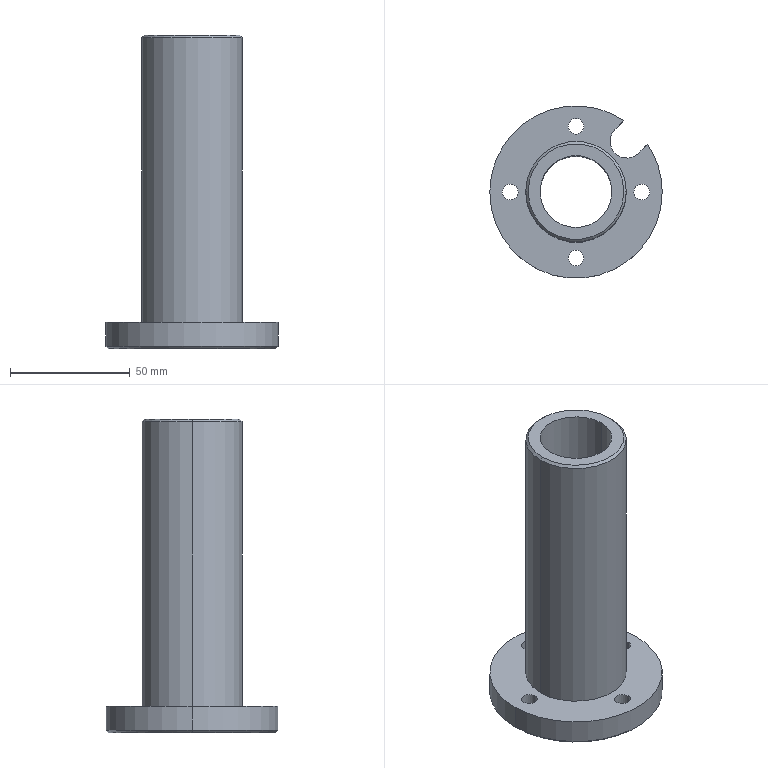Part | SolidWorks | features HoleWzd 2, Revolution 2, Chamfer 1, ICE 1 | 1 solid | 40 faces | box 72 x 72 x 131 mm | volume 113425 mm3 | cylinder 24 | plane 9 | cone 7 | commonest cylinder face diameters 6.6 x8 11 x8 72 x3 30 x2 42 x2 14 x1
STEP:
#1=CARTESIAN_POINT('',(-35.,0.,0.));
#2=VERTEX_POINT('',#1);
#3=CARTESIAN_POINT('',(19.299,29.198,0.));
#4=VERTEX_POINT('',#3);
#5=CARTESIAN_POINT('',(0.,0.,0.));
#6=DIRECTION('',(0.,0.,-1.));
#7=DIRECTION('',(-1.,0.,0.));
#8=AXIS2_PLACEMENT_3D('',#5,#6,#7);
#9=CIRCLE('',#8,35.);
#10=EDGE_CURVE('',#2,#4,#9,.T.);
#11=ORIENTED_EDGE('',*,*,#10,.F.);
#12=CARTESIAN_POINT('',(-36.,0.,1.));
#13=VERTEX_POINT('',#12);
#14=CARTESIAN_POINT('',(-35.,0.,0.));
#15=DIRECTION('',(-0.7071,0.,0.7071));
#16=VECTOR('',#15,1000.);
#17=LINE('',#14,#16);
#18=EDGE_CURVE('',#2,#13,#17,.T.);
#19=ORIENTED_EDGE('',*,*,#18,.T.);
#20=CARTESIAN_POINT('',(20.02,29.92,1.));
#21=VERTEX_POINT('',#20);
#22=CARTESIAN_POINT('',(0.,0.,1.));
#23=DIRECTION('',(0.,0.,1.));
#24=DIRECTION('',(-1.,0.,0.));
#25=AXIS2_PLACEMENT_3D('',#22,#23,#24);
#26=CIRCLE('',#25,36.);
#27=EDGE_CURVE('',#21,#13,#26,.T.);
#28=ORIENTED_EDGE('',*,*,#27,.F.);
#29=CARTESIAN_POINT('',(19.299,29.198,0.));
#30=CARTESIAN_POINT('',(19.539,29.439,0.3332));
#31=CARTESIAN_POINT('',(19.78,29.679,0.6666));
#32=CARTESIAN_POINT('',(20.02,29.92,1.));
#33=B_SPLINE_CURVE_WITH_KNOTS('',3,(#29,#30,#31,#32),.UNSPECIFIED.,.F.,.F.,(4,4),(0.,0.001428),.UNSPECIFIED.);
#34=EDGE_CURVE('',#4,#21,#33,.T.);
#35=ORIENTED_EDGE('',*,*,#34,.F.);
#36=EDGE_LOOP('',(#11,#19,#28,#35));
#37=FACE_OUTER_BOUND('',#36,.T.);
#38=CARTESIAN_POINT('',(0.,0.,0.));
#39=DIRECTION('',(0.,0.,1.));
#40=DIRECTION('',(1.,0.,0.));
#41=AXIS2_PLACEMENT_3D('',#38,#39,#40);
#42=CONICAL_SURFACE('',#41,35.,0.7854);
#43=ADVANCED_FACE('',(#37),#42,.T.);
#44=ORIENTED_EDGE('',*,*,#18,.F.);
#45=CARTESIAN_POINT('',(35.,0.,0.));
#46=VERTEX_POINT('',#45);
#47=CARTESIAN_POINT('',(0.,0.,0.));
#48=DIRECTION('',(0.,0.,-1.));
#49=DIRECTION('',(-1.,0.,0.));
#50=AXIS2_PLACEMENT_3D('',#47,#48,#49);
#51=CIRCLE('',#50,35.);
#52=EDGE_CURVE('',#46,#2,#51,.T.);
#53=ORIENTED_EDGE('',*,*,#52,.F.);
#54=CARTESIAN_POINT('',(36.,0.,1.));
#55=VERTEX_POINT('',#54);
#56=CARTESIAN_POINT('',(35.,0.,0.));
#57=DIRECTION('',(0.7071,0.,0.7071));
#58=VECTOR('',#57,1000.);
#59=LINE('',#56,#58);
#60=EDGE_CURVE('',#46,#55,#59,.T.);
#61=ORIENTED_EDGE('',*,*,#60,.T.);
#62=CARTESIAN_POINT('',(0.,0.,1.));
#63=DIRECTION('',(0.,0.,1.));
#64=DIRECTION('',(-1.,0.,0.));
#65=AXIS2_PLACEMENT_3D('',#62,#63,#64);
#66=CIRCLE('',#65,36.);
#67=EDGE_CURVE('',#13,#55,#66,.T.);
#68=ORIENTED_EDGE('',*,*,#67,.F.);
#69=EDGE_LOOP('',(#44,#53,#61,#68));
#70=FACE_OUTER_BOUND('',#69,.T.);
#71=CARTESIAN_POINT('',(0.,0.,0.));
#72=DIRECTION('',(0.,0.,1.));
#73=DIRECTION('',(1.,0.,0.));
#74=AXIS2_PLACEMENT_3D('',#71,#72,#73);
#75=CONICAL_SURFACE('',#74,35.,0.7854);
#76=ADVANCED_FACE('',(#70),#75,.T.);
#77=CARTESIAN_POINT('',(20.,0.,131.));
#78=VERTEX_POINT('',#77);
#79=CARTESIAN_POINT('',(-20.,0.,131.));
#80=VERTEX_POINT('',#79);
#81=CARTESIAN_POINT('',(0.,0.,131.));
#82=DIRECTION('',(0.,0.,1.));
#83=DIRECTION('',(1.,0.,0.));
#84=AXIS2_PLACEMENT_3D('',#81,#82,#83);
#85=CIRCLE('',#84,20.);
#86=EDGE_CURVE('',#78,#80,#85,.T.);
#87=ORIENTED_EDGE('',*,*,#86,.F.);
#88=CARTESIAN_POINT('',(21.,0.,130.));
#89=VERTEX_POINT('',#88);
#90=CARTESIAN_POINT('',(21.,0.,130.));
#91=DIRECTION('',(0.7071,0.,-0.7071));
#92=VECTOR('',#91,1000.);
#93=LINE('',#90,#92);
#94=EDGE_CURVE('',#78,#89,#93,.T.);
#95=ORIENTED_EDGE('',*,*,#94,.T.);
#96=CARTESIAN_POINT('',(-21.,0.,130.));
#97=VERTEX_POINT('',#96);
#98=CARTESIAN_POINT('',(0.,0.,130.));
#99=DIRECTION('',(0.,0.,-1.));
#100=DIRECTION('',(1.,0.,0.));
#101=AXIS2_PLACEMENT_3D('',#98,#99,#100);
#102=CIRCLE('',#101,21.);
#103=EDGE_CURVE('',#97,#89,#102,.T.);
#104=ORIENTED_EDGE('',*,*,#103,.F.);
#105=CARTESIAN_POINT('',(-21.,0.,130.));
#106=DIRECTION('',(-0.7071,0.,-0.7071));
#107=VECTOR('',#106,1000.);
#108=LINE('',#105,#107);
#109=EDGE_CURVE('',#80,#97,#108,.T.);
#110=ORIENTED_EDGE('',*,*,#109,.F.);
#111=EDGE_LOOP('',(#87,#95,#104,#110));
#112=FACE_OUTER_BOUND('',#111,.T.);
#113=CARTESIAN_POINT('',(0.,0.,130.));
#114=DIRECTION('',(0.,0.,-1.));
#115=DIRECTION('',(-1.,0.,0.));
#116=AXIS2_PLACEMENT_3D('',#113,#114,#115);
#117=CONICAL_SURFACE('',#116,21.,0.7854);
#118=ADVANCED_FACE('',(#112),#117,.T.);
#119=CARTESIAN_POINT('',(15.,0.,1.));
#120=VERTEX_POINT('',#119);
#121=CARTESIAN_POINT('',(-15.,0.,1.));
#122=VERTEX_POINT('',#121);
#123=CARTESIAN_POINT('',(0.,0.,1.));
#124=DIRECTION('',(0.,0.,-1.));
#125=DIRECTION('',(-1.,0.,0.));
#126=AXIS2_PLACEMENT_3D('',#123,#124,#125);
#127=CIRCLE('',#126,15.);
#128=EDGE_CURVE('',#120,#122,#127,.T.);
#129=ORIENTED_EDGE('',*,*,#128,.F.);
#130=CARTESIAN_POINT('',(16.,0.,0.));
#131=VERTEX_POINT('',#130);
#132=CARTESIAN_POINT('',(15.,0.,1.));
#133=DIRECTION('',(0.7071,0.,-0.7071));
#134=VECTOR('',#133,1000.);
#135=LINE('',#132,#134);
#136=EDGE_CURVE('',#120,#131,#135,.T.);
#137=ORIENTED_EDGE('',*,*,#136,.T.);
#138=CARTESIAN_POINT('',(-16.,0.,0.));
#139=VERTEX_POINT('',#138);
#140=CARTESIAN_POINT('',(0.,0.,0.));
#141=DIRECTION('',(0.,0.,1.));
#142=DIRECTION('',(-1.,0.,0.));
#143=AXIS2_PLACEMENT_3D('',#140,#141,#142);
#144=CIRCLE('',#143,16.);
#145=EDGE_CURVE('',#139,#131,#144,.T.);
#146=ORIENTED_EDGE('',*,*,#145,.F.);
#147=CARTESIAN_POINT('',(-15.,0.,1.));
#148=DIRECTION('',(-0.7071,0.,-0.7071));
#149=VECTOR('',#148,1000.);
#150=LINE('',#147,#149);
#151=EDGE_CURVE('',#122,#139,#150,.T.);
#152=ORIENTED_EDGE('',*,*,#151,.F.);
#153=EDGE_LOOP('',(#129,#137,#146,#152));
#154=FACE_OUTER_BOUND('',#153,.T.);
#155=CARTESIAN_POINT('',(0.,0.,1.));
#156=DIRECTION('',(0.,0.,-1.));
#157=DIRECTION('',(-1.,0.,0.));
#158=AXIS2_PLACEMENT_3D('',#155,#156,#157);
#159=CONICAL_SURFACE('',#158,15.,0.7854);
#160=ADVANCED_FACE('',(#154),#159,.F.);
#161=CARTESIAN_POINT('',(5.5,27.5,6.4));
#162=VERTEX_POINT('',#161);
#163=CARTESIAN_POINT('',(-5.5,27.5,6.4));
#164=VERTEX_POINT('',#163);
#165=CARTESIAN_POINT('',(0.,27.5,6.4));
#166=DIRECTION('',(0.,0.,-1.));
#167=DIRECTION('',(-1.,0.,0.));
#168=AXIS2_PLACEMENT_3D('',#165,#166,#167);
#169=CIRCLE('',#168,5.5);
#170=EDGE_CURVE('',#162,#164,#169,.T.);
#171=ORIENTED_EDGE('',*,*,#170,.F.);
#172=CARTESIAN_POINT('',(5.5,27.5,0.));
#173=VERTEX_POINT('',#172);
#174=CARTESIAN_POINT('',(5.5,27.5,0.));
#175=DIRECTION('',(0.,0.,-1.));
#176=VECTOR('',#175,1000.);
#177=LINE('',#174,#176);
#178=EDGE_CURVE('',#162,#173,#177,.T.);
#179=ORIENTED_EDGE('',*,*,#178,.T.);
#180=CARTESIAN_POINT('',(-5.5,27.5,0.));
#181=VERTEX_POINT('',#180);
#182=CARTESIAN_POINT('',(0.,27.5,0.));
#183=DIRECTION('',(0.,0.,-1.));
#184=DIRECTION('',(-1.,0.,0.));
#185=AXIS2_PLACEMENT_3D('',#182,#183,#184);
#186=CIRCLE('',#185,5.5);
#187=EDGE_CURVE('',#173,#181,#186,.T.);
#188=ORIENTED_EDGE('',*,*,#187,.T.);
#189=CARTESIAN_POINT('',(-5.5,27.5,0.));
#190=DIRECTION('',(0.,0.,-1.));
#191=VECTOR('',#190,1000.);
#192=LINE('',#189,#191);
#193=EDGE_CURVE('',#164,#181,#192,.T.);
#194=ORIENTED_EDGE('',*,*,#193,.F.);
#195=EDGE_LOOP('',(#171,#179,#188,#194));
#196=FACE_OUTER_BOUND('',#195,.T.);
#197=CARTESIAN_POINT('',(0.,27.5,0.));
#198=DIRECTION('',(0.,0.,-1.));
#199=DIRECTION('',(-1.,0.,0.));
#200=AXIS2_PLACEMENT_3D('',#197,#198,#199);
#201=CYLINDRICAL_SURFACE('',#200,5.5);
#202=ADVANCED_FACE('',(#196),#201,.F.);
#203=CARTESIAN_POINT('',(-3.3,27.5,11.));
#204=VERTEX_POINT('',#203);
#205=CARTESIAN_POINT('',(3.3,27.5,11.));
#206=VERTEX_POINT('',#205);
#207=CARTESIAN_POINT('',(0.,27.5,11.));
#208=DIRECTION('',(0.,0.,1.));
#209=DIRECTION('',(1.,0.,0.));
#210=AXIS2_PLACEMENT_3D('',#207,#208,#209);
#211=CIRCLE('',#210,3.3);
#212=EDGE_CURVE('',#204,#206,#211,.T.);
#213=ORIENTED_EDGE('',*,*,#212,.T.);
#214=CARTESIAN_POINT('',(3.3,27.5,6.4));
#215=VERTEX_POINT('',#214);
#216=CARTESIAN_POINT('',(3.3,27.5,0.));
#217=DIRECTION('',(0.,0.,-1.));
#218=VECTOR('',#217,1000.);
#219=LINE('',#216,#218);
#220=EDGE_CURVE('',#206,#215,#219,.T.);
#221=ORIENTED_EDGE('',*,*,#220,.T.);
#222=CARTESIAN_POINT('',(-3.3,27.5,6.4));
#223=VERTEX_POINT('',#222);
#224=CARTESIAN_POINT('',(0.,27.5,6.4));
#225=DIRECTION('',(0.,0.,-1.));
#226=DIRECTION('',(-1.,0.,0.));
#227=AXIS2_PLACEMENT_3D('',#224,#225,#226);
#228=CIRCLE('',#227,3.3);
#229=EDGE_CURVE('',#215,#223,#228,.T.);
#230=ORIENTED_EDGE('',*,*,#229,.T.);
#231=CARTESIAN_POINT('',(-3.3,27.5,0.));
#232=DIRECTION('',(0.,0.,-1.));
#233=VECTOR('',#232,1000.);
#234=LINE('',#231,#233);
#235=EDGE_CURVE('',#204,#223,#234,.T.);
#236=ORIENTED_EDGE('',*,*,#235,.F.);
#237=EDGE_LOOP('',(#213,#221,#230,#236));
#238=FACE_OUTER_BOUND('',#237,.T.);
#239=CARTESIAN_POINT('',(0.,27.5,0.));
#240=DIRECTION('',(0.,0.,-1.));
#241=DIRECTION('',(-1.,0.,0.));
#242=AXIS2_PLACEMENT_3D('',#239,#240,#241);
#243=CYLINDRICAL_SURFACE('',#242,3.3);
#244=ADVANCED_FACE('',(#238),#243,.F.);
#245=CARTESIAN_POINT('',(-22.,0.,6.4));
#246=VERTEX_POINT('',#245);
#247=CARTESIAN_POINT('',(-33.,0.,6.4));
#248=VERTEX_POINT('',#247);
#249=CARTESIAN_POINT('',(-27.5,0.,6.4));
#250=DIRECTION('',(0.,0.,-1.));
#251=DIRECTION('',(-1.,0.,0.));
#252=AXIS2_PLACEMENT_3D('',#249,#250,#251);
#253=CIRCLE('',#252,5.5);
#254=EDGE_CURVE('',#246,#248,#253,.T.);
#255=ORIENTED_EDGE('',*,*,#254,.F.);
#256=CARTESIAN_POINT('',(-22.,0.,0.));
#257=VERTEX_POINT('',#256);
#258=CARTESIAN_POINT('',(-22.,0.,0.));
#259=DIRECTION('',(0.,0.,-1.));
#260=VECTOR('',#259,1000.);
#261=LINE('',#258,#260);
#262=EDGE_CURVE('',#246,#257,#261,.T.);
#263=ORIENTED_EDGE('',*,*,#262,.T.);
#264=CARTESIAN_POINT('',(-33.,0.,0.));
#265=VERTEX_POINT('',#264);
#266=CARTESIAN_POINT('',(-27.5,0.,0.));
#267=DIRECTION('',(0.,0.,-1.));
#268=DIRECTION('',(-1.,0.,0.));
#269=AXIS2_PLACEMENT_3D('',#266,#267,#268);
#270=CIRCLE('',#269,5.5);
#271=EDGE_CURVE('',#257,#265,#270,.T.);
#272=ORIENTED_EDGE('',*,*,#271,.T.);
#273=CARTESIAN_POINT('',(-33.,0.,0.));
#274=DIRECTION('',(0.,0.,-1.));
#275=VECTOR('',#274,1000.);
#276=LINE('',#273,#275);
#277=EDGE_CURVE('',#248,#265,#276,.T.);
#278=ORIENTED_EDGE('',*,*,#277,.F.);
#279=EDGE_LOOP('',(#255,#263,#272,#278));
#280=FACE_OUTER_BOUND('',#279,.T.);
#281=CARTESIAN_POINT('',(-27.5,0.,0.));
#282=DIRECTION('',(0.,0.,-1.));
#283=DIRECTION('',(-1.,0.,0.));
#284=AXIS2_PLACEMENT_3D('',#281,#282,#283);
#285=CYLINDRICAL_SURFACE('',#284,5.5);
#286=ADVANCED_FACE('',(#280),#285,.F.);
#287=CARTESIAN_POINT('',(-30.8,0.,11.));
#288=VERTEX_POINT('',#287);
#289=CARTESIAN_POINT('',(-24.2,0.,11.));
#290=VERTEX_POINT('',#289);
#291=CARTESIAN_POINT('',(-27.5,0.,11.));
#292=DIRECTION('',(0.,0.,1.));
#293=DIRECTION('',(1.,0.,0.));
#294=AXIS2_PLACEMENT_3D('',#291,#292,#293);
#295=CIRCLE('',#294,3.3);
#296=EDGE_CURVE('',#288,#290,#295,.T.);
#297=ORIENTED_EDGE('',*,*,#296,.T.);
#298=CARTESIAN_POINT('',(-24.2,0.,6.4));
#299=VERTEX_POINT('',#298);
#300=CARTESIAN_POINT('',(-24.2,0.,0.));
#301=DIRECTION('',(0.,0.,-1.));
#302=VECTOR('',#301,1000.);
#303=LINE('',#300,#302);
#304=EDGE_CURVE('',#290,#299,#303,.T.);
#305=ORIENTED_EDGE('',*,*,#304,.T.);
#306=CARTESIAN_POINT('',(-30.8,0.,6.4));
#307=VERTEX_POINT('',#306);
#308=CARTESIAN_POINT('',(-27.5,0.,6.4));
#309=DIRECTION('',(0.,0.,-1.));
#310=DIRECTION('',(-1.,0.,0.));
#311=AXIS2_PLACEMENT_3D('',#308,#309,#310);
#312=CIRCLE('',#311,3.3);
#313=EDGE_CURVE('',#299,#307,#312,.T.);
#314=ORIENTED_EDGE('',*,*,#313,.T.);
#315=CARTESIAN_POINT('',(-30.8,0.,0.));
#316=DIRECTION('',(0.,0.,-1.));
#317=VECTOR('',#316,1000.);
#318=LINE('',#315,#317);
#319=EDGE_CURVE('',#288,#307,#318,.T.);
#320=ORIENTED_EDGE('',*,*,#319,.F.);
#321=EDGE_LOOP('',(#297,#305,#314,#320));
#322=FACE_OUTER_BOUND('',#321,.T.);
#323=CARTESIAN_POINT('',(-27.5,0.,0.));
#324=DIRECTION('',(0.,0.,-1.));
#325=DIRECTION('',(-1.,0.,0.));
#326=AXIS2_PLACEMENT_3D('',#323,#324,#325);
#327=CYLINDRICAL_SURFACE('',#326,3.3);
#328=ADVANCED_FACE('',(#322),#327,.F.);
#329=CARTESIAN_POINT('',(5.5,-27.5,6.4));
#330=VERTEX_POINT('',#329);
#331=CARTESIAN_POINT('',(-5.5,-27.5,6.4));
#332=VERTEX_POINT('',#331);
#333=CARTESIAN_POINT('',(0.,-27.5,6.4));
#334=DIRECTION('',(0.,0.,-1.));
#335=DIRECTION('',(-1.,0.,0.));
#336=AXIS2_PLACEMENT_3D('',#333,#334,#335);
#337=CIRCLE('',#336,5.5);
#338=EDGE_CURVE('',#330,#332,#337,.T.);
#339=ORIENTED_EDGE('',*,*,#338,.F.);
#340=CARTESIAN_POINT('',(5.5,-27.5,0.));
#341=VERTEX_POINT('',#340);
#342=CARTESIAN_POINT('',(5.5,-27.5,0.));
#343=DIRECTION('',(0.,0.,-1.));
#344=VECTOR('',#343,1000.);
#345=LINE('',#342,#344);
#346=EDGE_CURVE('',#330,#341,#345,.T.);
#347=ORIENTED_EDGE('',*,*,#346,.T.);
#348=CARTESIAN_POINT('',(-5.5,-27.5,0.));
#349=VERTEX_POINT('',#348);
#350=CARTESIAN_POINT('',(0.,-27.5,0.));
#351=DIRECTION('',(0.,0.,-1.));
#352=DIRECTION('',(-1.,0.,0.));
#353=AXIS2_PLACEMENT_3D('',#350,#351,#352);
#354=CIRCLE('',#353,5.5);
#355=EDGE_CURVE('',#341,#349,#354,.T.);
#356=ORIENTED_EDGE('',*,*,#355,.T.);
#357=CARTESIAN_POINT('',(-5.5,-27.5,0.));
#358=DIRECTION('',(0.,0.,-1.));
#359=VECTOR('',#358,1000.);
#360=LINE('',#357,#359);
#361=EDGE_CURVE('',#332,#349,#360,.T.);
#362=ORIENTED_EDGE('',*,*,#361,.F.);
#363=EDGE_LOOP('',(#339,#347,#356,#362));
#364=FACE_OUTER_BOUND('',#363,.T.);
#365=CARTESIAN_POINT('',(0.,-27.5,0.));
#366=DIRECTION('',(0.,0.,-1.));
#367=DIRECTION('',(-1.,0.,0.));
#368=AXIS2_PLACEMENT_3D('',#365,#366,#367);
#369=CYLINDRICAL_SURFACE('',#368,5.5);
#370=ADVANCED_FACE('',(#364),#369,.F.);
#371=CARTESIAN_POINT('',(-3.3,-27.5,11.));
#372=VERTEX_POINT('',#371);
#373=CARTESIAN_POINT('',(3.3,-27.5,11.));
#374=VERTEX_POINT('',#373);
#375=CARTESIAN_POINT('',(0.,-27.5,11.));
#376=DIRECTION('',(0.,0.,1.));
#377=DIRECTION('',(1.,0.,0.));
#378=AXIS2_PLACEMENT_3D('',#375,#376,#377);
#379=CIRCLE('',#378,3.3);
#380=EDGE_CURVE('',#372,#374,#379,.T.);
#381=ORIENTED_EDGE('',*,*,#380,.T.);
#382=CARTESIAN_POINT('',(3.3,-27.5,6.4));
#383=VERTEX_POINT('',#382);
#384=CARTESIAN_POINT('',(3.3,-27.5,0.));
#385=DIRECTION('',(0.,0.,-1.));
#386=VECTOR('',#385,1000.);
#387=LINE('',#384,#386);
#388=EDGE_CURVE('',#374,#383,#387,.T.);
#389=ORIENTED_EDGE('',*,*,#388,.T.);
#390=CARTESIAN_POINT('',(-3.3,-27.5,6.4));
#391=VERTEX_POINT('',#390);
#392=CARTESIAN_POINT('',(0.,-27.5,6.4));
#393=DIRECTION('',(0.,0.,-1.));
#394=DIRECTION('',(-1.,0.,0.));
#395=AXIS2_PLACEMENT_3D('',#392,#393,#394);
#396=CIRCLE('',#395,3.3);
#397=EDGE_CURVE('',#383,#391,#396,.T.);
#398=ORIENTED_EDGE('',*,*,#397,.T.);
#399=CARTESIAN_POINT('',(-3.3,-27.5,0.));
#400=DIRECTION('',(0.,0.,-1.));
#401=VECTOR('',#400,1000.);
#402=LINE('',#399,#401);
#403=EDGE_CURVE('',#372,#391,#402,.T.);
#404=ORIENTED_EDGE('',*,*,#403,.F.);
#405=EDGE_LOOP('',(#381,#389,#398,#404));
#406=FACE_OUTER_BOUND('',#405,.T.);
#407=CARTESIAN_POINT('',(0.,-27.5,0.));
#408=DIRECTION('',(0.,0.,-1.));
#409=DIRECTION('',(-1.,0.,0.));
#410=AXIS2_PLACEMENT_3D('',#407,#408,#409);
#411=CYLINDRICAL_SURFACE('',#410,3.3);
#412=ADVANCED_FACE('',(#406),#411,.F.);
#413=CARTESIAN_POINT('',(33.,0.,6.4));
#414=VERTEX_POINT('',#413);
#415=CARTESIAN_POINT('',(22.,0.,6.4));
#416=VERTEX_POINT('',#415);
#417=CARTESIAN_POINT('',(27.5,0.,6.4));
#418=DIRECTION('',(0.,0.,-1.));
#419=DIRECTION('',(-1.,0.,0.));
#420=AXIS2_PLACEMENT_3D('',#417,#418,#419);
#421=CIRCLE('',#420,5.5);
#422=EDGE_CURVE('',#414,#416,#421,.T.);
#423=ORIENTED_EDGE('',*,*,#422,.F.);
#424=CARTESIAN_POINT('',(33.,0.,0.));
#425=VERTEX_POINT('',#424);
#426=CARTESIAN_POINT('',(33.,0.,0.));
#427=DIRECTION('',(0.,0.,-1.));
#428=VECTOR('',#427,1000.);
#429=LINE('',#426,#428);
#430=EDGE_CURVE('',#414,#425,#429,.T.);
#431=ORIENTED_EDGE('',*,*,#430,.T.);
#432=CARTESIAN_POINT('',(22.,0.,0.));
#433=VERTEX_POINT('',#432);
#434=CARTESIAN_POINT('',(27.5,0.,0.));
#435=DIRECTION('',(0.,0.,-1.));
#436=DIRECTION('',(-1.,0.,0.));
#437=AXIS2_PLACEMENT_3D('',#434,#435,#436);
#438=CIRCLE('',#437,5.5);
#439=EDGE_CURVE('',#425,#433,#438,.T.);
#440=ORIENTED_EDGE('',*,*,#439,.T.);
#441=CARTESIAN_POINT('',(22.,0.,0.));
#442=DIRECTION('',(0.,0.,-1.));
#443=VECTOR('',#442,1000.);
#444=LINE('',#441,#443);
#445=EDGE_CURVE('',#416,#433,#444,.T.);
#446=ORIENTED_EDGE('',*,*,#445,.F.);
#447=EDGE_LOOP('',(#423,#431,#440,#446));
#448=FACE_OUTER_BOUND('',#447,.T.);
#449=CARTESIAN_POINT('',(27.5,0.,0.));
#450=DIRECTION('',(0.,0.,-1.));
#451=DIRECTION('',(-1.,0.,0.));
#452=AXIS2_PLACEMENT_3D('',#449,#450,#451);
#453=CYLINDRICAL_SURFACE('',#452,5.5);
#454=ADVANCED_FACE('',(#448),#453,.F.);
#455=CARTESIAN_POINT('',(24.2,0.,11.));
#456=VERTEX_POINT('',#455);
#457=CARTESIAN_POINT('',(30.8,0.,11.));
#458=VERTEX_POINT('',#457);
#459=CARTESIAN_POINT('',(27.5,0.,11.));
#460=DIRECTION('',(0.,0.,1.));
#461=DIRECTION('',(1.,0.,0.));
#462=AXIS2_PLACEMENT_3D('',#459,#460,#461);
#463=CIRCLE('',#462,3.3);
#464=EDGE_CURVE('',#456,#458,#463,.T.);
#465=ORIENTED_EDGE('',*,*,#464,.T.);
#466=CARTESIAN_POINT('',(30.8,0.,6.4));
#467=VERTEX_POINT('',#466);
#468=CARTESIAN_POINT('',(30.8,0.,0.));
#469=DIRECTION('',(0.,0.,-1.));
#470=VECTOR('',#469,1000.);
#471=LINE('',#468,#470);
#472=EDGE_CURVE('',#458,#467,#471,.T.);
#473=ORIENTED_EDGE('',*,*,#472,.T.);
#474=CARTESIAN_POINT('',(24.2,0.,6.4));
#475=VERTEX_POINT('',#474);
#476=CARTESIAN_POINT('',(27.5,0.,6.4));
#477=DIRECTION('',(0.,0.,-1.));
#478=DIRECTION('',(-1.,0.,0.));
#479=AXIS2_PLACEMENT_3D('',#476,#477,#478);
#480=CIRCLE('',#479,3.3);
#481=EDGE_CURVE('',#467,#475,#480,.T.);
#482=ORIENTED_EDGE('',*,*,#481,.T.);
#483=CARTESIAN_POINT('',(24.2,0.,0.));
#484=DIRECTION('',(0.,0.,-1.));
#485=VECTOR('',#484,1000.);
#486=LINE('',#483,#485);
#487=EDGE_CURVE('',#456,#475,#486,.T.);
#488=ORIENTED_EDGE('',*,*,#487,.F.);
#489=EDGE_LOOP('',(#465,#473,#482,#488));
#490=FACE_OUTER_BOUND('',#489,.T.);
#491=CARTESIAN_POINT('',(27.5,0.,0.));
#492=DIRECTION('',(0.,0.,-1.));
#493=DIRECTION('',(-1.,0.,0.));
#494=AXIS2_PLACEMENT_3D('',#491,#492,#493);
#495=CYLINDRICAL_SURFACE('',#494,3.3);
#496=ADVANCED_FACE('',(#490),#495,.F.);
#497=CARTESIAN_POINT('',(15.,0.,131.));
#498=VERTEX_POINT('',#497);
#499=CARTESIAN_POINT('',(-15.,0.,131.));
#500=VERTEX_POINT('',#499);
#501=CARTESIAN_POINT('',(0.,0.,131.));
#502=DIRECTION('',(0.,0.,-1.));
#503=DIRECTION('',(-1.,0.,0.));
#504=AXIS2_PLACEMENT_3D('',#501,#502,#503);
#505=CIRCLE('',#504,15.);
#506=EDGE_CURVE('',#498,#500,#505,.T.);
#507=ORIENTED_EDGE('',*,*,#506,.F.);
#508=CARTESIAN_POINT('',(15.,0.,0.));
#509=DIRECTION('',(0.,0.,-1.));
#510=VECTOR('',#509,1000.);
#511=LINE('',#508,#510);
#512=EDGE_CURVE('',#498,#120,#511,.T.);
#513=ORIENTED_EDGE('',*,*,#512,.T.);
#514=ORIENTED_EDGE('',*,*,#128,.T.);
#515=CARTESIAN_POINT('',(-15.,0.,0.));
#516=DIRECTION('',(0.,0.,-1.));
#517=VECTOR('',#516,1000.);
#518=LINE('',#515,#517);
#519=EDGE_CURVE('',#500,#122,#518,.T.);
#520=ORIENTED_EDGE('',*,*,#519,.F.);
#521=EDGE_LOOP('',(#507,#513,#514,#520));
#522=FACE_OUTER_BOUND('',#521,.T.);
#523=CARTESIAN_POINT('',(0.,0.,0.));
#524=DIRECTION('',(0.,0.,-1.));
#525=DIRECTION('',(-1.,0.,0.));
#526=AXIS2_PLACEMENT_3D('',#523,#524,#525);
#527=CYLINDRICAL_SURFACE('',#526,15.);
#528=ADVANCED_FACE('',(#522),#527,.F.);
#529=ORIENTED_EDGE('',*,*,#103,.T.);
#530=CARTESIAN_POINT('',(21.,0.,11.));
#531=VERTEX_POINT('',#530);
#532=CARTESIAN_POINT('',(21.,0.,131.));
#533=DIRECTION('',(0.,0.,-1.));
#534=VECTOR('',#533,1000.);
#535=LINE('',#532,#534);
#536=EDGE_CURVE('',#89,#531,#535,.T.);
#537=ORIENTED_EDGE('',*,*,#536,.T.);
#538=CARTESIAN_POINT('',(-21.,0.,11.));
#539=VERTEX_POINT('',#538);
#540=CARTESIAN_POINT('',(0.,0.,11.));
#541=DIRECTION('',(0.,0.,1.));
#542=DIRECTION('',(1.,0.,0.));
#543=AXIS2_PLACEMENT_3D('',#540,#541,#542);
#544=CIRCLE('',#543,21.);
#545=EDGE_CURVE('',#531,#539,#544,.T.);
#546=ORIENTED_EDGE('',*,*,#545,.T.);
#547=CARTESIAN_POINT('',(-21.,0.,131.));
#548=DIRECTION('',(0.,0.,-1.));
#549=VECTOR('',#548,1000.);
#550=LINE('',#547,#549);
#551=EDGE_CURVE('',#97,#539,#550,.T.);
#552=ORIENTED_EDGE('',*,*,#551,.F.);
#553=EDGE_LOOP('',(#529,#537,#546,#552));
#554=FACE_OUTER_BOUND('',#553,.T.);
#555=CARTESIAN_POINT('',(0.,0.,131.));
#556=DIRECTION('',(0.,0.,-1.));
#557=DIRECTION('',(-1.,0.,0.));
#558=AXIS2_PLACEMENT_3D('',#555,#556,#557);
#559=CYLINDRICAL_SURFACE('',#558,21.);
#560=ADVANCED_FACE('',(#554),#559,.T.);
#561=CARTESIAN_POINT('',(29.92,20.02,11.));
#562=VERTEX_POINT('',#561);
#563=CARTESIAN_POINT('',(36.,0.,11.));
#564=VERTEX_POINT('',#563);
#565=CARTESIAN_POINT('',(0.,0.,11.));
#566=DIRECTION('',(0.,0.,-1.));
#567=DIRECTION('',(-1.,0.,0.));
#568=AXIS2_PLACEMENT_3D('',#565,#566,#567);
#569=CIRCLE('',#568,36.);
#570=EDGE_CURVE('',#562,#564,#569,.T.);
#571=ORIENTED_EDGE('',*,*,#570,.T.);
#572=CARTESIAN_POINT('',(36.,0.,11.));
#573=DIRECTION('',(0.,0.,-1.));
#574=VECTOR('',#573,1000.);
#575=LINE('',#572,#574);
#576=EDGE_CURVE('',#564,#55,#575,.T.);
#577=ORIENTED_EDGE('',*,*,#576,.T.);
#578=CARTESIAN_POINT('',(29.92,20.02,1.));
#579=VERTEX_POINT('',#578);
#580=CARTESIAN_POINT('',(0.,0.,1.));
#581=DIRECTION('',(0.,0.,1.));
#582=DIRECTION('',(-1.,0.,0.));
#583=AXIS2_PLACEMENT_3D('',#580,#581,#582);
#584=CIRCLE('',#583,36.);
#585=EDGE_CURVE('',#55,#579,#584,.T.);
#586=ORIENTED_EDGE('',*,*,#585,.T.);
#587=CARTESIAN_POINT('',(29.92,20.02,0.));
#588=DIRECTION('',(0.,0.,1.));
#589=VECTOR('',#588,1000.);
#590=LINE('',#587,#589);
#591=EDGE_CURVE('',#579,#562,#590,.T.);
#592=ORIENTED_EDGE('',*,*,#591,.T.);
#593=EDGE_LOOP('',(#571,#577,#586,#592));
#594=FACE_OUTER_BOUND('',#593,.T.);
#595=CARTESIAN_POINT('',(0.,0.,11.));
#596=DIRECTION('',(0.,0.,-1.));
#597=DIRECTION('',(-1.,0.,0.));
#598=AXIS2_PLACEMENT_3D('',#595,#596,#597);
#599=CYLINDRICAL_SURFACE('',#598,36.);
#600=ADVANCED_FACE('',(#594),#599,.T.);
#601=ORIENTED_EDGE('',*,*,#576,.F.);
#602=CARTESIAN_POINT('',(-36.,0.,11.));
#603=VERTEX_POINT('',#602);
#604=CARTESIAN_POINT('',(0.,0.,11.));
#605=DIRECTION('',(0.,0.,-1.));
#606=DIRECTION('',(-1.,0.,0.));
#607=AXIS2_PLACEMENT_3D('',#604,#605,#606);
#608=CIRCLE('',#607,36.);
#609=EDGE_CURVE('',#564,#603,#608,.T.);
#610=ORIENTED_EDGE('',*,*,#609,.T.);
#611=CARTESIAN_POINT('',(-36.,0.,11.));
#612=DIRECTION('',(0.,0.,-1.));
#613=VECTOR('',#612,1000.);
#614=LINE('',#611,#613);
#615=EDGE_CURVE('',#603,#13,#614,.T.);
#616=ORIENTED_EDGE('',*,*,#615,.T.);
#617=ORIENTED_EDGE('',*,*,#67,.T.);
#618=EDGE_LOOP('',(#601,#610,#616,#617));
#619=FACE_OUTER_BOUND('',#618,.T.);
#620=CARTESIAN_POINT('',(0.,0.,11.));
#621=DIRECTION('',(0.,0.,-1.));
#622=DIRECTION('',(-1.,0.,0.));
#623=AXIS2_PLACEMENT_3D('',#620,#621,#622);
#624=CYLINDRICAL_SURFACE('',#623,36.);
#625=ADVANCED_FACE('',(#619),#624,.T.);
#626=CARTESIAN_POINT('',(0.,0.,131.));
#627=DIRECTION('',(0.,0.,1.));
#628=DIRECTION('',(1.,0.,0.));
#629=AXIS2_PLACEMENT_3D('',#626,#627,#628);
#630=CIRCLE('',#629,20.);
#631=EDGE_CURVE('',#80,#78,#630,.T.);
#632=ORIENTED_EDGE('',*,*,#631,.T.);
#633=ORIENTED_EDGE('',*,*,#86,.T.);
#634=EDGE_LOOP('',(#632,#633));
#635=FACE_OUTER_BOUND('',#634,.T.);
#636=CARTESIAN_POINT('',(0.,0.,131.));
#637=DIRECTION('',(0.,0.,-1.));
#638=DIRECTION('',(-1.,0.,0.));
#639=AXIS2_PLACEMENT_3D('',#636,#637,#638);
#640=CIRCLE('',#639,15.);
#641=EDGE_CURVE('',#500,#498,#640,.T.);
#642=ORIENTED_EDGE('',*,*,#641,.T.);
#643=ORIENTED_EDGE('',*,*,#506,.T.);
#644=EDGE_LOOP('',(#642,#643));
#645=FACE_BOUND('',#644,.T.);
#646=CARTESIAN_POINT('',(21.,0.,131.));
#647=DIRECTION('',(0.,0.,1.));
#648=DIRECTION('',(1.,0.,0.));
#649=AXIS2_PLACEMENT_3D('',#646,#647,#648);
#650=PLANE('',#649);
#651=ADVANCED_FACE('',(#635,#645),#650,.T.);
#652=ORIENTED_EDGE('',*,*,#615,.F.);
#653=CARTESIAN_POINT('',(20.02,29.92,11.));
#654=VERTEX_POINT('',#653);
#655=CARTESIAN_POINT('',(0.,0.,11.));
#656=DIRECTION('',(0.,0.,-1.));
#657=DIRECTION('',(-1.,0.,0.));
#658=AXIS2_PLACEMENT_3D('',#655,#656,#657);
#659=CIRCLE('',#658,36.);
#660=EDGE_CURVE('',#603,#654,#659,.T.);
#661=ORIENTED_EDGE('',*,*,#660,.T.);
#662=CARTESIAN_POINT('',(20.02,29.92,0.));
#663=DIRECTION('',(0.,0.,1.));
#664=VECTOR('',#663,1000.);
#665=LINE('',#662,#664);
#666=EDGE_CURVE('',#21,#654,#665,.T.);
#667=ORIENTED_EDGE('',*,*,#666,.F.);
#668=ORIENTED_EDGE('',*,*,#27,.T.);
#669=EDGE_LOOP('',(#652,#661,#667,#668));
#670=FACE_OUTER_BOUND('',#669,.T.);
#671=CARTESIAN_POINT('',(0.,0.,11.));
#672=DIRECTION('',(0.,0.,-1.));
#673=DIRECTION('',(-1.,0.,0.));
#674=AXIS2_PLACEMENT_3D('',#671,#672,#673);
#675=CYLINDRICAL_SURFACE('',#674,36.);
#676=ADVANCED_FACE('',(#670),#675,.T.);
#677=ORIENTED_EDGE('',*,*,#212,.F.);
#678=CARTESIAN_POINT('',(0.,27.5,11.));
#679=DIRECTION('',(0.,0.,1.));
#680=DIRECTION('',(1.,0.,0.));
#681=AXIS2_PLACEMENT_3D('',#678,#679,#680);
#682=CIRCLE('',#681,3.3);
#683=EDGE_CURVE('',#206,#204,#682,.T.);
#684=ORIENTED_EDGE('',*,*,#683,.F.);
#685=EDGE_LOOP('',(#677,#684));
#686=FACE_BOUND('',#685,.T.);
#687=ORIENTED_EDGE('',*,*,#296,.F.);
#688=CARTESIAN_POINT('',(-27.5,0.,11.));
#689=DIRECTION('',(0.,0.,1.));
#690=DIRECTION('',(1.,0.,0.));
#691=AXIS2_PLACEMENT_3D('',#688,#689,#690);
#692=CIRCLE('',#691,3.3);
#693=EDGE_CURVE('',#290,#288,#692,.T.);
#694=ORIENTED_EDGE('',*,*,#693,.F.);
#695=EDGE_LOOP('',(#687,#694));
#696=FACE_BOUND('',#695,.T.);
#697=ORIENTED_EDGE('',*,*,#380,.F.);
#698=CARTESIAN_POINT('',(0.,-27.5,11.));
#699=DIRECTION('',(0.,0.,1.));
#700=DIRECTION('',(1.,0.,0.));
#701=AXIS2_PLACEMENT_3D('',#698,#699,#700);
#702=CIRCLE('',#701,3.3);
#703=EDGE_CURVE('',#374,#372,#702,.T.);
#704=ORIENTED_EDGE('',*,*,#703,.F.);
#705=EDGE_LOOP('',(#697,#704));
#706=FACE_BOUND('',#705,.T.);
#707=ORIENTED_EDGE('',*,*,#464,.F.);
#708=CARTESIAN_POINT('',(27.5,0.,11.));
#709=DIRECTION('',(0.,0.,1.));
#710=DIRECTION('',(1.,0.,0.));
#711=AXIS2_PLACEMENT_3D('',#708,#709,#710);
#712=CIRCLE('',#711,3.3);
#713=EDGE_CURVE('',#458,#456,#712,.T.);
#714=ORIENTED_EDGE('',*,*,#713,.F.);
#715=EDGE_LOOP('',(#707,#714));
#716=FACE_BOUND('',#715,.T.);
#717=CARTESIAN_POINT('',(0.,0.,11.));
#718=DIRECTION('',(0.,0.,1.));
#719=DIRECTION('',(1.,0.,0.));
#720=AXIS2_PLACEMENT_3D('',#717,#718,#719);
#721=CIRCLE('',#720,21.);
#722=EDGE_CURVE('',#539,#531,#721,.T.);
#723=ORIENTED_EDGE('',*,*,#722,.F.);
#724=ORIENTED_EDGE('',*,*,#545,.F.);
#725=EDGE_LOOP('',(#723,#724));
#726=FACE_BOUND('',#725,.T.);
#727=CARTESIAN_POINT('',(26.163,16.263,11.));
#728=VERTEX_POINT('',#727);
#729=CARTESIAN_POINT('',(26.163,16.263,11.));
#730=DIRECTION('',(0.7071,0.7071,0.));
#731=VECTOR('',#730,1000.);
#732=LINE('',#729,#731);
#733=EDGE_CURVE('',#728,#562,#732,.T.);
#734=ORIENTED_EDGE('',*,*,#733,.F.);
#735=CARTESIAN_POINT('',(16.263,26.163,11.));
#736=VERTEX_POINT('',#735);
#737=CARTESIAN_POINT('',(21.213,21.213,11.));
#738=DIRECTION('',(0.,0.,1.));
#739=DIRECTION('',(1.,0.,0.));
#740=AXIS2_PLACEMENT_3D('',#737,#738,#739);
#741=CIRCLE('',#740,7.);
#742=EDGE_CURVE('',#736,#728,#741,.T.);
#743=ORIENTED_EDGE('',*,*,#742,.F.);
#744=CARTESIAN_POINT('',(20.02,29.92,11.));
#745=DIRECTION('',(-0.7071,-0.7071,0.));
#746=VECTOR('',#745,1000.);
#747=LINE('',#744,#746);
#748=EDGE_CURVE('',#654,#736,#747,.T.);
#749=ORIENTED_EDGE('',*,*,#748,.F.);
#750=ORIENTED_EDGE('',*,*,#660,.F.);
#751=ORIENTED_EDGE('',*,*,#609,.F.);
#752=ORIENTED_EDGE('',*,*,#570,.F.);
#753=EDGE_LOOP('',(#734,#743,#749,#750,#751,#752));
#754=FACE_OUTER_BOUND('',#753,.T.);
#755=CARTESIAN_POINT('',(36.,0.,11.));
#756=DIRECTION('',(0.,0.,1.));
#757=DIRECTION('',(1.,0.,0.));
#758=AXIS2_PLACEMENT_3D('',#755,#756,#757);
#759=PLANE('',#758);
#760=ADVANCED_FACE('',(#686,#696,#706,#716,#726,#754),#759,.T.);
#761=ORIENTED_EDGE('',*,*,#145,.T.);
#762=CARTESIAN_POINT('',(0.,0.,0.));
#763=DIRECTION('',(0.,0.,1.));
#764=DIRECTION('',(-1.,0.,0.));
#765=AXIS2_PLACEMENT_3D('',#762,#763,#764);
#766=CIRCLE('',#765,16.);
#767=EDGE_CURVE('',#131,#139,#766,.T.);
#768=ORIENTED_EDGE('',*,*,#767,.T.);
#769=EDGE_LOOP('',(#761,#768));
#770=FACE_BOUND('',#769,.T.);
#771=CARTESIAN_POINT('',(0.,27.5,0.));
#772=DIRECTION('',(0.,0.,-1.));
#773=DIRECTION('',(-1.,0.,0.));
#774=AXIS2_PLACEMENT_3D('',#771,#772,#773);
#775=CIRCLE('',#774,5.5);
#776=EDGE_CURVE('',#181,#173,#775,.T.);
#777=ORIENTED_EDGE('',*,*,#776,.F.);
#778=ORIENTED_EDGE('',*,*,#187,.F.);
#779=EDGE_LOOP('',(#777,#778));
#780=FACE_BOUND('',#779,.T.);
#781=CARTESIAN_POINT('',(-27.5,0.,0.));
#782=DIRECTION('',(0.,0.,-1.));
#783=DIRECTION('',(-1.,0.,0.));
#784=AXIS2_PLACEMENT_3D('',#781,#782,#783);
#785=CIRCLE('',#784,5.5);
#786=EDGE_CURVE('',#265,#257,#785,.T.);
#787=ORIENTED_EDGE('',*,*,#786,.F.);
#788=ORIENTED_EDGE('',*,*,#271,.F.);
#789=EDGE_LOOP('',(#787,#788));
#790=FACE_BOUND('',#789,.T.);
#791=CARTESIAN_POINT('',(0.,-27.5,0.));
#792=DIRECTION('',(0.,0.,-1.));
#793=DIRECTION('',(-1.,0.,0.));
#794=AXIS2_PLACEMENT_3D('',#791,#792,#793);
#795=CIRCLE('',#794,5.5);
#796=EDGE_CURVE('',#349,#341,#795,.T.);
#797=ORIENTED_EDGE('',*,*,#796,.F.);
#798=ORIENTED_EDGE('',*,*,#355,.F.);
#799=EDGE_LOOP('',(#797,#798));
#800=FACE_BOUND('',#799,.T.);
#801=CARTESIAN_POINT('',(27.5,0.,0.));
#802=DIRECTION('',(0.,0.,-1.));
#803=DIRECTION('',(-1.,0.,0.));
#804=AXIS2_PLACEMENT_3D('',#801,#802,#803);
#805=CIRCLE('',#804,5.5);
#806=EDGE_CURVE('',#433,#425,#805,.T.);
#807=ORIENTED_EDGE('',*,*,#806,.F.);
#808=ORIENTED_EDGE('',*,*,#439,.F.);
#809=EDGE_LOOP('',(#807,#808));
#810=FACE_BOUND('',#809,.T.);
#811=CARTESIAN_POINT('',(26.163,16.263,0.));
#812=VERTEX_POINT('',#811);
#813=CARTESIAN_POINT('',(29.198,19.299,0.));
#814=VERTEX_POINT('',#813);
#815=CARTESIAN_POINT('',(26.163,16.263,0.));
#816=DIRECTION('',(0.7071,0.7071,0.));
#817=VECTOR('',#816,1000.);
#818=LINE('',#815,#817);
#819=EDGE_CURVE('',#812,#814,#818,.T.);
#820=ORIENTED_EDGE('',*,*,#819,.T.);
#821=CARTESIAN_POINT('',(0.,0.,0.));
#822=DIRECTION('',(0.,0.,-1.));
#823=DIRECTION('',(-1.,0.,0.));
#824=AXIS2_PLACEMENT_3D('',#821,#822,#823);
#825=CIRCLE('',#824,35.);
#826=EDGE_CURVE('',#814,#46,#825,.T.);
#827=ORIENTED_EDGE('',*,*,#826,.T.);
#828=ORIENTED_EDGE('',*,*,#52,.T.);
#829=ORIENTED_EDGE('',*,*,#10,.T.);
#830=CARTESIAN_POINT('',(16.263,26.163,0.));
#831=VERTEX_POINT('',#830);
#832=CARTESIAN_POINT('',(20.02,29.92,0.));
#833=DIRECTION('',(-0.7071,-0.7071,0.));
#834=VECTOR('',#833,1000.);
#835=LINE('',#832,#834);
#836=EDGE_CURVE('',#4,#831,#835,.T.);
#837=ORIENTED_EDGE('',*,*,#836,.T.);
#838=CARTESIAN_POINT('',(21.213,21.213,0.));
#839=DIRECTION('',(0.,0.,1.));
#840=DIRECTION('',(1.,0.,0.));
#841=AXIS2_PLACEMENT_3D('',#838,#839,#840);
#842=CIRCLE('',#841,7.);
#843=EDGE_CURVE('',#831,#812,#842,.T.);
#844=ORIENTED_EDGE('',*,*,#843,.T.);
#845=EDGE_LOOP('',(#820,#827,#828,#829,#837,#844));
#846=FACE_OUTER_BOUND('',#845,.T.);
#847=CARTESIAN_POINT('',(0.,0.,0.));
#848=DIRECTION('',(0.,0.,-1.));
#849=DIRECTION('',(-1.,0.,0.));
#850=AXIS2_PLACEMENT_3D('',#847,#848,#849);
#851=PLANE('',#850);
#852=ADVANCED_FACE('',(#770,#780,#790,#800,#810,#846),#851,.T.);
#853=ORIENTED_EDGE('',*,*,#591,.F.);
#854=CARTESIAN_POINT('',(29.92,20.02,1.));
#855=CARTESIAN_POINT('',(29.679,19.78,0.6666));
#856=CARTESIAN_POINT('',(29.439,19.539,0.3332));
#857=CARTESIAN_POINT('',(29.198,19.299,0.));
#858=B_SPLINE_CURVE_WITH_KNOTS('',3,(#854,#855,#856,#857),.UNSPECIFIED.,.F.,.F.,(4,4),(0.,0.001428),.UNSPECIFIED.);
#859=EDGE_CURVE('',#579,#814,#858,.T.);
#860=ORIENTED_EDGE('',*,*,#859,.T.);
#861=ORIENTED_EDGE('',*,*,#819,.F.);
#862=CARTESIAN_POINT('',(26.163,16.263,0.));
#863=DIRECTION('',(0.,0.,1.));
#864=VECTOR('',#863,1000.);
#865=LINE('',#862,#864);
#866=EDGE_CURVE('',#812,#728,#865,.T.);
#867=ORIENTED_EDGE('',*,*,#866,.T.);
#868=ORIENTED_EDGE('',*,*,#733,.T.);
#869=EDGE_LOOP('',(#853,#860,#861,#867,#868));
#870=FACE_OUTER_BOUND('',#869,.T.);
#871=CARTESIAN_POINT('',(26.163,16.263,0.));
#872=DIRECTION('',(0.7071,-0.7071,0.));
#873=DIRECTION('',(0.7071,0.7071,0.));
#874=AXIS2_PLACEMENT_3D('',#871,#872,#873);
#875=PLANE('',#874);
#876=ADVANCED_FACE('',(#870),#875,.F.);
#877=ORIENTED_EDGE('',*,*,#742,.T.);
#878=ORIENTED_EDGE('',*,*,#866,.F.);
#879=ORIENTED_EDGE('',*,*,#843,.F.);
#880=CARTESIAN_POINT('',(16.263,26.163,0.));
#881=DIRECTION('',(0.,0.,1.));
#882=VECTOR('',#881,1000.);
#883=LINE('',#880,#882);
#884=EDGE_CURVE('',#831,#736,#883,.T.);
#885=ORIENTED_EDGE('',*,*,#884,.T.);
#886=EDGE_LOOP('',(#877,#878,#879,#885));
#887=FACE_OUTER_BOUND('',#886,.T.);
#888=CARTESIAN_POINT('',(21.213,21.213,0.));
#889=DIRECTION('',(0.,0.,1.));
#890=DIRECTION('',(1.,0.,0.));
#891=AXIS2_PLACEMENT_3D('',#888,#889,#890);
#892=CYLINDRICAL_SURFACE('',#891,7.);
#893=ADVANCED_FACE('',(#887),#892,.F.);
#894=ORIENTED_EDGE('',*,*,#836,.F.);
#895=ORIENTED_EDGE('',*,*,#34,.T.);
#896=ORIENTED_EDGE('',*,*,#666,.T.);
#897=ORIENTED_EDGE('',*,*,#748,.T.);
#898=ORIENTED_EDGE('',*,*,#884,.F.);
#899=EDGE_LOOP('',(#894,#895,#896,#897,#898));
#900=FACE_OUTER_BOUND('',#899,.T.);
#901=CARTESIAN_POINT('',(20.02,29.92,0.));
#902=DIRECTION('',(-0.7071,0.7071,0.));
#903=DIRECTION('',(-0.7071,-0.7071,0.));
#904=AXIS2_PLACEMENT_3D('',#901,#902,#903);
#905=PLANE('',#904);
#906=ADVANCED_FACE('',(#900),#905,.F.);
#907=ORIENTED_EDGE('',*,*,#536,.F.);
#908=CARTESIAN_POINT('',(0.,0.,130.));
#909=DIRECTION('',(0.,0.,-1.));
#910=DIRECTION('',(1.,0.,0.));
#911=AXIS2_PLACEMENT_3D('',#908,#909,#910);
#912=CIRCLE('',#911,21.);
#913=EDGE_CURVE('',#89,#97,#912,.T.);
#914=ORIENTED_EDGE('',*,*,#913,.T.);
#915=ORIENTED_EDGE('',*,*,#551,.T.);
#916=ORIENTED_EDGE('',*,*,#722,.T.);
#917=EDGE_LOOP('',(#907,#914,#915,#916));
#918=FACE_OUTER_BOUND('',#917,.T.);
#919=CARTESIAN_POINT('',(0.,0.,131.));
#920=DIRECTION('',(0.,0.,-1.));
#921=DIRECTION('',(-1.,0.,0.));
#922=AXIS2_PLACEMENT_3D('',#919,#920,#921);
#923=CYLINDRICAL_SURFACE('',#922,21.);
#924=ADVANCED_FACE('',(#918),#923,.T.);
#925=ORIENTED_EDGE('',*,*,#512,.F.);
#926=ORIENTED_EDGE('',*,*,#641,.F.);
#927=ORIENTED_EDGE('',*,*,#519,.T.);
#928=CARTESIAN_POINT('',(0.,0.,1.));
#929=DIRECTION('',(0.,0.,-1.));
#930=DIRECTION('',(-1.,0.,0.));
#931=AXIS2_PLACEMENT_3D('',#928,#929,#930);
#932=CIRCLE('',#931,15.);
#933=EDGE_CURVE('',#122,#120,#932,.T.);
#934=ORIENTED_EDGE('',*,*,#933,.T.);
#935=EDGE_LOOP('',(#925,#926,#927,#934));
#936=FACE_OUTER_BOUND('',#935,.T.);
#937=CARTESIAN_POINT('',(0.,0.,0.));
#938=DIRECTION('',(0.,0.,-1.));
#939=DIRECTION('',(-1.,0.,0.));
#940=AXIS2_PLACEMENT_3D('',#937,#938,#939);
#941=CYLINDRICAL_SURFACE('',#940,15.);
#942=ADVANCED_FACE('',(#936),#941,.F.);
#943=ORIENTED_EDGE('',*,*,#472,.F.);
#944=ORIENTED_EDGE('',*,*,#713,.T.);
#945=ORIENTED_EDGE('',*,*,#487,.T.);
#946=CARTESIAN_POINT('',(27.5,0.,6.4));
#947=DIRECTION('',(0.,0.,-1.));
#948=DIRECTION('',(-1.,0.,0.));
#949=AXIS2_PLACEMENT_3D('',#946,#947,#948);
#950=CIRCLE('',#949,3.3);
#951=EDGE_CURVE('',#475,#467,#950,.T.);
#952=ORIENTED_EDGE('',*,*,#951,.T.);
#953=EDGE_LOOP('',(#943,#944,#945,#952));
#954=FACE_OUTER_BOUND('',#953,.T.);
#955=CARTESIAN_POINT('',(27.5,0.,0.));
#956=DIRECTION('',(0.,0.,-1.));
#957=DIRECTION('',(-1.,0.,0.));
#958=AXIS2_PLACEMENT_3D('',#955,#956,#957);
#959=CYLINDRICAL_SURFACE('',#958,3.3);
#960=ADVANCED_FACE('',(#954),#959,.F.);
#961=ORIENTED_EDGE('',*,*,#951,.F.);
#962=ORIENTED_EDGE('',*,*,#481,.F.);
#963=EDGE_LOOP('',(#961,#962));
#964=FACE_BOUND('',#963,.T.);
#965=CARTESIAN_POINT('',(27.5,0.,6.4));
#966=DIRECTION('',(0.,0.,-1.));
#967=DIRECTION('',(-1.,0.,0.));
#968=AXIS2_PLACEMENT_3D('',#965,#966,#967);
#969=CIRCLE('',#968,5.5);
#970=EDGE_CURVE('',#416,#414,#969,.T.);
#971=ORIENTED_EDGE('',*,*,#970,.T.);
#972=ORIENTED_EDGE('',*,*,#422,.T.);
#973=EDGE_LOOP('',(#971,#972));
#974=FACE_OUTER_BOUND('',#973,.T.);
#975=CARTESIAN_POINT('',(30.8,0.,6.4));
#976=DIRECTION('',(0.,0.,1.));
#977=DIRECTION('',(1.,0.,0.));
#978=AXIS2_PLACEMENT_3D('',#975,#976,#977);
#979=PLANE('',#978);
#980=ADVANCED_FACE('',(#964,#974),#979,.F.);
#981=ORIENTED_EDGE('',*,*,#430,.F.);
#982=ORIENTED_EDGE('',*,*,#970,.F.);
#983=ORIENTED_EDGE('',*,*,#445,.T.);
#984=ORIENTED_EDGE('',*,*,#806,.T.);
#985=EDGE_LOOP('',(#981,#982,#983,#984));
#986=FACE_OUTER_BOUND('',#985,.T.);
#987=CARTESIAN_POINT('',(27.5,0.,0.));
#988=DIRECTION('',(0.,0.,-1.));
#989=DIRECTION('',(-1.,0.,0.));
#990=AXIS2_PLACEMENT_3D('',#987,#988,#989);
#991=CYLINDRICAL_SURFACE('',#990,5.5);
#992=ADVANCED_FACE('',(#986),#991,.F.);
#993=ORIENTED_EDGE('',*,*,#388,.F.);
#994=ORIENTED_EDGE('',*,*,#703,.T.);
#995=ORIENTED_EDGE('',*,*,#403,.T.);
#996=CARTESIAN_POINT('',(0.,-27.5,6.4));
#997=DIRECTION('',(0.,0.,-1.));
#998=DIRECTION('',(-1.,0.,0.));
#999=AXIS2_PLACEMENT_3D('',#996,#997,#998);
#1000=CIRCLE('',#999,3.3);
#1001=EDGE_CURVE('',#391,#383,#1000,.T.);
#1002=ORIENTED_EDGE('',*,*,#1001,.T.);
#1003=EDGE_LOOP('',(#993,#994,#995,#1002));
#1004=FACE_OUTER_BOUND('',#1003,.T.);
#1005=CARTESIAN_POINT('',(0.,-27.5,0.));
#1006=DIRECTION('',(0.,0.,-1.));
#1007=DIRECTION('',(-1.,0.,0.));
#1008=AXIS2_PLACEMENT_3D('',#1005,#1006,#1007);
#1009=CYLINDRICAL_SURFACE('',#1008,3.3);
#1010=ADVANCED_FACE('',(#1004),#1009,.F.);
#1011=ORIENTED_EDGE('',*,*,#1001,.F.);
#1012=ORIENTED_EDGE('',*,*,#397,.F.);
#1013=EDGE_LOOP('',(#1011,#1012));
#1014=FACE_BOUND('',#1013,.T.);
#1015=CARTESIAN_POINT('',(0.,-27.5,6.4));
#1016=DIRECTION('',(0.,0.,-1.));
#1017=DIRECTION('',(-1.,0.,0.));
#1018=AXIS2_PLACEMENT_3D('',#1015,#1016,#1017);
#1019=CIRCLE('',#1018,5.5);
#1020=EDGE_CURVE('',#332,#330,#1019,.T.);
#1021=ORIENTED_EDGE('',*,*,#1020,.T.);
#1022=ORIENTED_EDGE('',*,*,#338,.T.);
#1023=EDGE_LOOP('',(#1021,#1022));
#1024=FACE_OUTER_BOUND('',#1023,.T.);
#1025=CARTESIAN_POINT('',(3.3,-27.5,6.4));
#1026=DIRECTION('',(0.,0.,1.));
#1027=DIRECTION('',(1.,0.,0.));
#1028=AXIS2_PLACEMENT_3D('',#1025,#1026,#1027);
#1029=PLANE('',#1028);
#1030=ADVANCED_FACE('',(#1014,#1024),#1029,.F.);
#1031=ORIENTED_EDGE('',*,*,#346,.F.);
#1032=ORIENTED_EDGE('',*,*,#1020,.F.);
#1033=ORIENTED_EDGE('',*,*,#361,.T.);
#1034=ORIENTED_EDGE('',*,*,#796,.T.);
#1035=EDGE_LOOP('',(#1031,#1032,#1033,#1034));
#1036=FACE_OUTER_BOUND('',#1035,.T.);
#1037=CARTESIAN_POINT('',(0.,-27.5,0.));
#1038=DIRECTION('',(0.,0.,-1.));
#1039=DIRECTION('',(-1.,0.,0.));
#1040=AXIS2_PLACEMENT_3D('',#1037,#1038,#1039);
#1041=CYLINDRICAL_SURFACE('',#1040,5.5);
#1042=ADVANCED_FACE('',(#1036),#1041,.F.);
#1043=ORIENTED_EDGE('',*,*,#304,.F.);
#1044=ORIENTED_EDGE('',*,*,#693,.T.);
#1045=ORIENTED_EDGE('',*,*,#319,.T.);
#1046=CARTESIAN_POINT('',(-27.5,0.,6.4));
#1047=DIRECTION('',(0.,0.,-1.));
#1048=DIRECTION('',(-1.,0.,0.));
#1049=AXIS2_PLACEMENT_3D('',#1046,#1047,#1048);
#1050=CIRCLE('',#1049,3.3);
#1051=EDGE_CURVE('',#307,#299,#1050,.T.);
#1052=ORIENTED_EDGE('',*,*,#1051,.T.);
#1053=EDGE_LOOP('',(#1043,#1044,#1045,#1052));
#1054=FACE_OUTER_BOUND('',#1053,.T.);
#1055=CARTESIAN_POINT('',(-27.5,0.,0.));
#1056=DIRECTION('',(0.,0.,-1.));
#1057=DIRECTION('',(-1.,0.,0.));
#1058=AXIS2_PLACEMENT_3D('',#1055,#1056,#1057);
#1059=CYLINDRICAL_SURFACE('',#1058,3.3);
#1060=ADVANCED_FACE('',(#1054),#1059,.F.);
#1061=ORIENTED_EDGE('',*,*,#1051,.F.);
#1062=ORIENTED_EDGE('',*,*,#313,.F.);
#1063=EDGE_LOOP('',(#1061,#1062));
#1064=FACE_BOUND('',#1063,.T.);
#1065=CARTESIAN_POINT('',(-27.5,0.,6.4));
#1066=DIRECTION('',(0.,0.,-1.));
#1067=DIRECTION('',(-1.,0.,0.));
#1068=AXIS2_PLACEMENT_3D('',#1065,#1066,#1067);
#1069=CIRCLE('',#1068,5.5);
#1070=EDGE_CURVE('',#248,#246,#1069,.T.);
#1071=ORIENTED_EDGE('',*,*,#1070,.T.);
#1072=ORIENTED_EDGE('',*,*,#254,.T.);
#1073=EDGE_LOOP('',(#1071,#1072));
#1074=FACE_OUTER_BOUND('',#1073,.T.);
#1075=CARTESIAN_POINT('',(-24.2,0.,6.4));
#1076=DIRECTION('',(0.,0.,1.));
#1077=DIRECTION('',(1.,0.,0.));
#1078=AXIS2_PLACEMENT_3D('',#1075,#1076,#1077);
#1079=PLANE('',#1078);
#1080=ADVANCED_FACE('',(#1064,#1074),#1079,.F.);
#1081=ORIENTED_EDGE('',*,*,#262,.F.);
#1082=ORIENTED_EDGE('',*,*,#1070,.F.);
#1083=ORIENTED_EDGE('',*,*,#277,.T.);
#1084=ORIENTED_EDGE('',*,*,#786,.T.);
#1085=EDGE_LOOP('',(#1081,#1082,#1083,#1084));
#1086=FACE_OUTER_BOUND('',#1085,.T.);
#1087=CARTESIAN_POINT('',(-27.5,0.,0.));
#1088=DIRECTION('',(0.,0.,-1.));
#1089=DIRECTION('',(-1.,0.,0.));
#1090=AXIS2_PLACEMENT_3D('',#1087,#1088,#1089);
#1091=CYLINDRICAL_SURFACE('',#1090,5.5);
#1092=ADVANCED_FACE('',(#1086),#1091,.F.);
#1093=ORIENTED_EDGE('',*,*,#220,.F.);
#1094=ORIENTED_EDGE('',*,*,#683,.T.);
#1095=ORIENTED_EDGE('',*,*,#235,.T.);
#1096=CARTESIAN_POINT('',(0.,27.5,6.4));
#1097=DIRECTION('',(0.,0.,-1.));
#1098=DIRECTION('',(-1.,0.,0.));
#1099=AXIS2_PLACEMENT_3D('',#1096,#1097,#1098);
#1100=CIRCLE('',#1099,3.3);
#1101=EDGE_CURVE('',#223,#215,#1100,.T.);
#1102=ORIENTED_EDGE('',*,*,#1101,.T.);
#1103=EDGE_LOOP('',(#1093,#1094,#1095,#1102));
#1104=FACE_OUTER_BOUND('',#1103,.T.);
#1105=CARTESIAN_POINT('',(0.,27.5,0.));
#1106=DIRECTION('',(0.,0.,-1.));
#1107=DIRECTION('',(-1.,0.,0.));
#1108=AXIS2_PLACEMENT_3D('',#1105,#1106,#1107);
#1109=CYLINDRICAL_SURFACE('',#1108,3.3);
#1110=ADVANCED_FACE('',(#1104),#1109,.F.);
#1111=ORIENTED_EDGE('',*,*,#1101,.F.);
#1112=ORIENTED_EDGE('',*,*,#229,.F.);
#1113=EDGE_LOOP('',(#1111,#1112));
#1114=FACE_BOUND('',#1113,.T.);
#1115=CARTESIAN_POINT('',(0.,27.5,6.4));
#1116=DIRECTION('',(0.,0.,-1.));
#1117=DIRECTION('',(-1.,0.,0.));
#1118=AXIS2_PLACEMENT_3D('',#1115,#1116,#1117);
#1119=CIRCLE('',#1118,5.5);
#1120=EDGE_CURVE('',#164,#162,#1119,.T.);
#1121=ORIENTED_EDGE('',*,*,#1120,.T.);
#1122=ORIENTED_EDGE('',*,*,#170,.T.);
#1123=EDGE_LOOP('',(#1121,#1122));
#1124=FACE_OUTER_BOUND('',#1123,.T.);
#1125=CARTESIAN_POINT('',(3.3,27.5,6.4));
#1126=DIRECTION('',(0.,0.,1.));
#1127=DIRECTION('',(1.,0.,0.));
#1128=AXIS2_PLACEMENT_3D('',#1125,#1126,#1127);
#1129=PLANE('',#1128);
#1130=ADVANCED_FACE('',(#1114,#1124),#1129,.F.);
#1131=ORIENTED_EDGE('',*,*,#178,.F.);
#1132=ORIENTED_EDGE('',*,*,#1120,.F.);
#1133=ORIENTED_EDGE('',*,*,#193,.T.);
#1134=ORIENTED_EDGE('',*,*,#776,.T.);
#1135=EDGE_LOOP('',(#1131,#1132,#1133,#1134));
#1136=FACE_OUTER_BOUND('',#1135,.T.);
#1137=CARTESIAN_POINT('',(0.,27.5,0.));
#1138=DIRECTION('',(0.,0.,-1.));
#1139=DIRECTION('',(-1.,0.,0.));
#1140=AXIS2_PLACEMENT_3D('',#1137,#1138,#1139);
#1141=CYLINDRICAL_SURFACE('',#1140,5.5);
#1142=ADVANCED_FACE('',(#1136),#1141,.F.);
#1143=ORIENTED_EDGE('',*,*,#136,.F.);
#1144=ORIENTED_EDGE('',*,*,#933,.F.);
#1145=ORIENTED_EDGE('',*,*,#151,.T.);
#1146=ORIENTED_EDGE('',*,*,#767,.F.);
#1147=EDGE_LOOP('',(#1143,#1144,#1145,#1146));
#1148=FACE_OUTER_BOUND('',#1147,.T.);
#1149=CARTESIAN_POINT('',(0.,0.,1.));
#1150=DIRECTION('',(0.,0.,-1.));
#1151=DIRECTION('',(-1.,0.,0.));
#1152=AXIS2_PLACEMENT_3D('',#1149,#1150,#1151);
#1153=CONICAL_SURFACE('',#1152,15.,0.7854);
#1154=ADVANCED_FACE('',(#1148),#1153,.F.);
#1155=ORIENTED_EDGE('',*,*,#94,.F.);
#1156=ORIENTED_EDGE('',*,*,#631,.F.);
#1157=ORIENTED_EDGE('',*,*,#109,.T.);
#1158=ORIENTED_EDGE('',*,*,#913,.F.);
#1159=EDGE_LOOP('',(#1155,#1156,#1157,#1158));
#1160=FACE_OUTER_BOUND('',#1159,.T.);
#1161=CARTESIAN_POINT('',(0.,0.,130.));
#1162=DIRECTION('',(0.,0.,-1.));
#1163=DIRECTION('',(-1.,0.,0.));
#1164=AXIS2_PLACEMENT_3D('',#1161,#1162,#1163);
#1165=CONICAL_SURFACE('',#1164,21.,0.7854);
#1166=ADVANCED_FACE('',(#1160),#1165,.T.);
#1167=ORIENTED_EDGE('',*,*,#60,.F.);
#1168=ORIENTED_EDGE('',*,*,#826,.F.);
#1169=ORIENTED_EDGE('',*,*,#859,.F.);
#1170=ORIENTED_EDGE('',*,*,#585,.F.);
#1171=EDGE_LOOP('',(#1167,#1168,#1169,#1170));
#1172=FACE_OUTER_BOUND('',#1171,.T.);
#1173=CARTESIAN_POINT('',(0.,0.,0.));
#1174=DIRECTION('',(0.,0.,1.));
#1175=DIRECTION('',(1.,0.,0.));
#1176=AXIS2_PLACEMENT_3D('',#1173,#1174,#1175);
#1177=CONICAL_SURFACE('',#1176,35.,0.7854);
#1178=ADVANCED_FACE('',(#1172),#1177,.T.);
#1179=CLOSED_SHELL('',(#43,#76,#118,#160,#202,#244,#286,#328,#370,#412,#454,#496,#528,#560,#600,#625,#651,#676,#760,#852,#876,#893,#906,#924,#942,#960,#980,#992,#1010,#1030,#1042,#1060,#1080,#1092,#1110,#1130,#1142,#1154,#1166,#1178));
#1180=MANIFOLD_SOLID_BREP('',#1179);
#1181=CARTESIAN_POINT('',(0.,0.,0.));
#1182=DIRECTION('',(0.,0.,1.));
#1183=DIRECTION('',(1.,0.,0.));
#1184=AXIS2_PLACEMENT_3D('',#1181,#1182,#1183);
#1185=(LENGTH_UNIT()NAMED_UNIT(*)SI_UNIT(.MILLI.,.METRE.));
#1186=UNCERTAINTY_MEASURE_WITH_UNIT(LENGTH_MEASURE(0.00001),#1185,'','');
#1187=(NAMED_UNIT(*)PLANE_ANGLE_UNIT()SI_UNIT($,.RADIAN.));
#1188=(NAMED_UNIT(*)SI_UNIT($,.STERADIAN.)SOLID_ANGLE_UNIT());
#1189=(GEOMETRIC_REPRESENTATION_CONTEXT(3)GLOBAL_UNCERTAINTY_ASSIGNED_CONTEXT((#1186))GLOBAL_UNIT_ASSIGNED_CONTEXT((#1185,#1187,#1188))REPRESENTATION_CONTEXT('',''));
#1190=ADVANCED_BREP_SHAPE_REPRESENTATION('',(#1180,#1184),#1189);